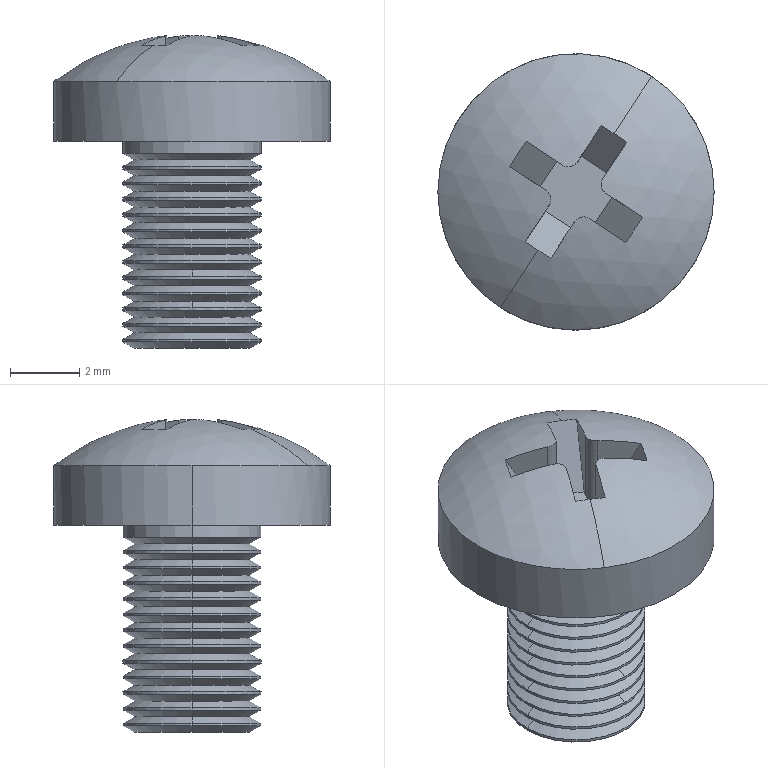Part | SolidWorks | features BaseBody 1 | 1 solid | 100 faces | box 8 x 8 x 9.057 mm | volume 179.133 mm3 | cone 50 | cylinder 33 | plane 15 | sphere 2 | commonest cylinder face diameters 4 x26 0.6 x5 8 x2